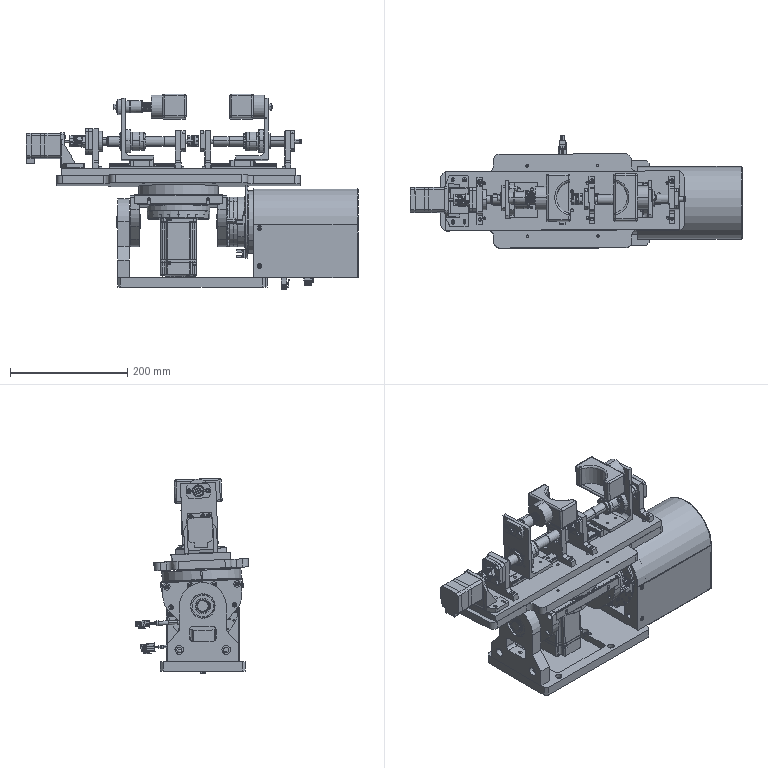Part | SolidWorks | features CompositeCurve 2, ReferencePattern 2, MirrorCompFeat 1 | 219 solids | 10117 faces | volume 4755058 mm3 | plane 4343 | cylinder 3844 | cone 1049 | spline 325 | sphere 300 | torus 256 | commonest cylinder face diameters 0.4 x318 5.5 x296 2.5 x264 6 x259 3.5 x220 1 x149